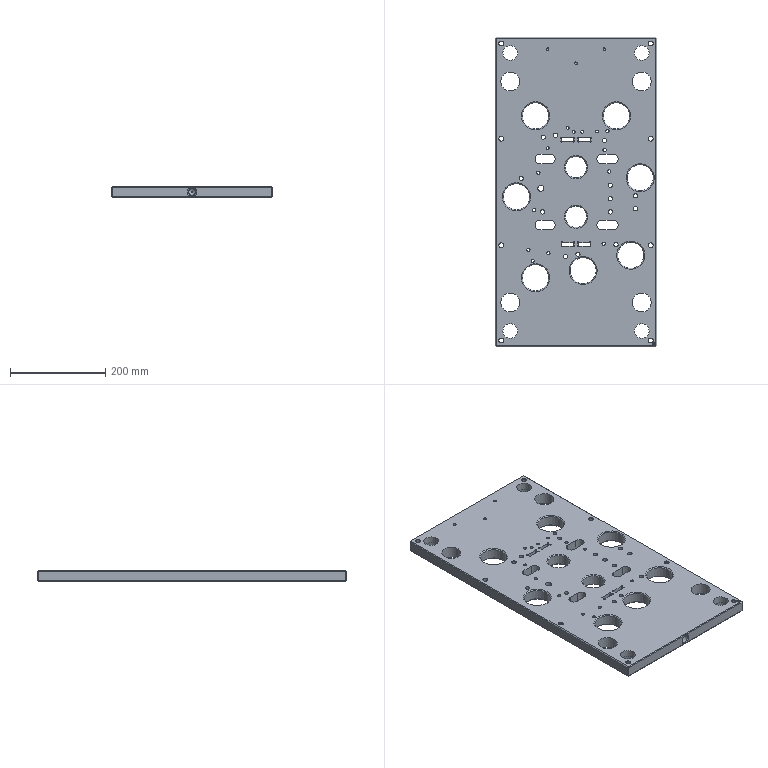Part | STEP file | P011002B002-000 | 1 solid | 2096 faces | box 340 x 650 x 25 mm | volume 4617723 mm3 | plane 1178 | other 701 | cylinder 167 | cone 50 | commonest cylinder face diameters 3 x44 9 x13 14 x13 7 x9 11 x9 6 x8